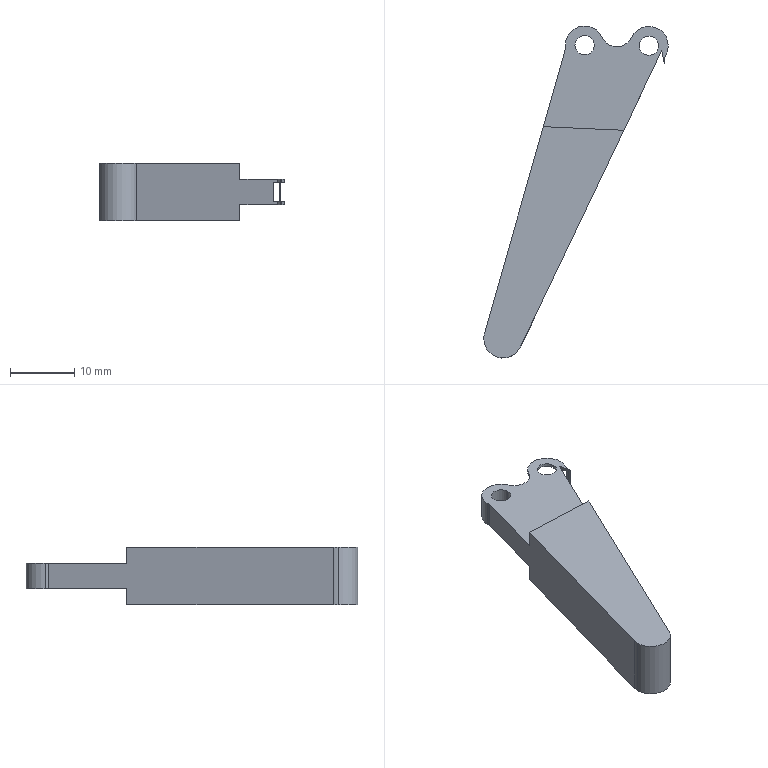Part | SolidWorks | features ICE 2, Extrusion 1, MirrorPattern 1, Scale 1 | 1 solid | 29 faces | box 28.674 x 51.63 x 9 mm | volume 3668 mm3 | cylinder 15 | plane 14 | commonest cylinder face diameters 3 x6 6 x6 4 x2 5 x1
STEP:
#1=CARTESIAN_POINT('',(-17.174,-2.918,4.));
#2=VERTEX_POINT('',#1);
#3=CARTESIAN_POINT('',(-17.133,-3.412,4.));
#4=VERTEX_POINT('',#3);
#5=CARTESIAN_POINT('',(-14.174,-2.918,4.));
#6=DIRECTION('',(0.,0.,1.));
#7=DIRECTION('',(1.,0.,0.));
#8=AXIS2_PLACEMENT_3D('',#5,#6,#7);
#9=CIRCLE('',#8,3.);
#10=EDGE_CURVE('',#2,#4,#9,.T.);
#11=ORIENTED_EDGE('',*,*,#10,.F.);
#12=CARTESIAN_POINT('',(-17.174,-2.918,0.));
#13=VERTEX_POINT('',#12);
#14=CARTESIAN_POINT('',(-17.174,-2.918,4.));
#15=DIRECTION('',(0.,0.,-1.));
#16=VECTOR('',#15,1000.);
#17=LINE('',#14,#16);
#18=EDGE_CURVE('',#2,#13,#17,.T.);
#19=ORIENTED_EDGE('',*,*,#18,.T.);
#20=CARTESIAN_POINT('',(-17.133,-3.412,0.));
#21=VERTEX_POINT('',#20);
#22=CARTESIAN_POINT('',(-14.174,-2.918,0.));
#23=DIRECTION('',(0.,0.,1.));
#24=DIRECTION('',(1.,0.,0.));
#25=AXIS2_PLACEMENT_3D('',#22,#23,#24);
#26=CIRCLE('',#25,3.);
#27=EDGE_CURVE('',#13,#21,#26,.T.);
#28=ORIENTED_EDGE('',*,*,#27,.T.);
#29=CARTESIAN_POINT('',(-17.133,-3.412,4.));
#30=DIRECTION('',(0.,0.,-1.));
#31=VECTOR('',#30,1000.);
#32=LINE('',#29,#31);
#33=EDGE_CURVE('',#4,#21,#32,.T.);
#34=ORIENTED_EDGE('',*,*,#33,.F.);
#35=EDGE_LOOP('',(#11,#19,#28,#34));
#36=FACE_OUTER_BOUND('',#35,.T.);
#37=CARTESIAN_POINT('',(-14.174,-2.918,4.));
#38=DIRECTION('',(0.,0.,-1.));
#39=DIRECTION('',(-1.,0.,0.));
#40=AXIS2_PLACEMENT_3D('',#37,#38,#39);
#41=CYLINDRICAL_SURFACE('',#40,3.);
#42=ADVANCED_FACE('',(#36),#41,.T.);
#43=CARTESIAN_POINT('',(-15.674,-2.918,4.));
#44=VERTEX_POINT('',#43);
#45=CARTESIAN_POINT('',(-12.674,-2.918,4.));
#46=VERTEX_POINT('',#45);
#47=CARTESIAN_POINT('',(-14.174,-2.918,4.));
#48=DIRECTION('',(0.,0.,1.));
#49=DIRECTION('',(1.,0.,0.));
#50=AXIS2_PLACEMENT_3D('',#47,#48,#49);
#51=CIRCLE('',#50,1.5);
#52=EDGE_CURVE('',#44,#46,#51,.T.);
#53=ORIENTED_EDGE('',*,*,#52,.T.);
#54=CARTESIAN_POINT('',(-12.674,-2.918,0.));
#55=VERTEX_POINT('',#54);
#56=CARTESIAN_POINT('',(-12.674,-2.918,4.));
#57=DIRECTION('',(0.,0.,-1.));
#58=VECTOR('',#57,1000.);
#59=LINE('',#56,#58);
#60=EDGE_CURVE('',#46,#55,#59,.T.);
#61=ORIENTED_EDGE('',*,*,#60,.T.);
#62=CARTESIAN_POINT('',(-15.674,-2.918,0.));
#63=VERTEX_POINT('',#62);
#64=CARTESIAN_POINT('',(-14.174,-2.918,0.));
#65=DIRECTION('',(0.,0.,1.));
#66=DIRECTION('',(1.,0.,0.));
#67=AXIS2_PLACEMENT_3D('',#64,#65,#66);
#68=CIRCLE('',#67,1.5);
#69=EDGE_CURVE('',#63,#55,#68,.T.);
#70=ORIENTED_EDGE('',*,*,#69,.F.);
#71=CARTESIAN_POINT('',(-15.674,-2.918,4.));
#72=DIRECTION('',(0.,0.,-1.));
#73=VECTOR('',#72,1000.);
#74=LINE('',#71,#73);
#75=EDGE_CURVE('',#44,#63,#74,.T.);
#76=ORIENTED_EDGE('',*,*,#75,.F.);
#77=EDGE_LOOP('',(#53,#61,#70,#76));
#78=FACE_OUTER_BOUND('',#77,.T.);
#79=CARTESIAN_POINT('',(-14.174,-2.918,4.));
#80=DIRECTION('',(0.,0.,-1.));
#81=DIRECTION('',(-1.,0.,0.));
#82=AXIS2_PLACEMENT_3D('',#79,#80,#81);
#83=CYLINDRICAL_SURFACE('',#82,1.5);
#84=ADVANCED_FACE('',(#78),#83,.F.);
#85=CARTESIAN_POINT('',(-29.848,-48.547,6.5));
#86=VERTEX_POINT('',#85);
#87=CARTESIAN_POINT('',(-24.14,-49.838,6.5));
#88=VERTEX_POINT('',#87);
#89=CARTESIAN_POINT('',(-26.848,-48.547,6.5));
#90=DIRECTION('',(0.,0.,1.));
#91=DIRECTION('',(1.,0.,0.));
#92=AXIS2_PLACEMENT_3D('',#89,#90,#91);
#93=CIRCLE('',#92,3.);
#94=EDGE_CURVE('',#86,#88,#93,.T.);
#95=ORIENTED_EDGE('',*,*,#94,.F.);
#96=CARTESIAN_POINT('',(-29.848,-48.547,-2.5));
#97=VERTEX_POINT('',#96);
#98=CARTESIAN_POINT('',(-29.848,-48.547,4.));
#99=DIRECTION('',(0.,0.,-1.));
#100=VECTOR('',#99,1000.);
#101=LINE('',#98,#100);
#102=EDGE_CURVE('',#86,#97,#101,.T.);
#103=ORIENTED_EDGE('',*,*,#102,.T.);
#104=CARTESIAN_POINT('',(-24.14,-49.838,-2.5));
#105=VERTEX_POINT('',#104);
#106=CARTESIAN_POINT('',(-26.848,-48.547,-2.5));
#107=DIRECTION('',(0.,0.,1.));
#108=DIRECTION('',(1.,0.,0.));
#109=AXIS2_PLACEMENT_3D('',#106,#107,#108);
#110=CIRCLE('',#109,3.);
#111=EDGE_CURVE('',#97,#105,#110,.T.);
#112=ORIENTED_EDGE('',*,*,#111,.T.);
#113=CARTESIAN_POINT('',(-24.14,-49.838,4.));
#114=DIRECTION('',(0.,0.,-1.));
#115=VECTOR('',#114,1000.);
#116=LINE('',#113,#115);
#117=EDGE_CURVE('',#88,#105,#116,.T.);
#118=ORIENTED_EDGE('',*,*,#117,.F.);
#119=EDGE_LOOP('',(#95,#103,#112,#118));
#120=FACE_OUTER_BOUND('',#119,.T.);
#121=CARTESIAN_POINT('',(-26.848,-48.547,4.));
#122=DIRECTION('',(0.,0.,-1.));
#123=DIRECTION('',(-1.,0.,0.));
#124=AXIS2_PLACEMENT_3D('',#121,#122,#123);
#125=CYLINDRICAL_SURFACE('',#124,3.);
#126=ADVANCED_FACE('',(#120),#125,.T.);
#127=CARTESIAN_POINT('',(-5.674,-2.989,0.5));
#128=VERTEX_POINT('',#127);
#129=CARTESIAN_POINT('',(-2.674,-2.989,0.5));
#130=VERTEX_POINT('',#129);
#131=CARTESIAN_POINT('',(-4.174,-2.989,0.5));
#132=DIRECTION('',(0.,0.,1.));
#133=DIRECTION('',(1.,0.,0.));
#134=AXIS2_PLACEMENT_3D('',#131,#132,#133);
#135=CIRCLE('',#134,1.5);
#136=EDGE_CURVE('',#128,#130,#135,.T.);
#137=ORIENTED_EDGE('',*,*,#136,.T.);
#138=CARTESIAN_POINT('',(-2.674,-2.989,0.));
#139=VERTEX_POINT('',#138);
#140=CARTESIAN_POINT('',(-2.674,-2.989,4.));
#141=DIRECTION('',(0.,0.,-1.));
#142=VECTOR('',#141,1000.);
#143=LINE('',#140,#142);
#144=EDGE_CURVE('',#130,#139,#143,.T.);
#145=ORIENTED_EDGE('',*,*,#144,.T.);
#146=CARTESIAN_POINT('',(-5.674,-2.989,0.));
#147=VERTEX_POINT('',#146);
#148=CARTESIAN_POINT('',(-4.174,-2.989,0.));
#149=DIRECTION('',(0.,0.,1.));
#150=DIRECTION('',(1.,0.,0.));
#151=AXIS2_PLACEMENT_3D('',#148,#149,#150);
#152=CIRCLE('',#151,1.5);
#153=EDGE_CURVE('',#147,#139,#152,.T.);
#154=ORIENTED_EDGE('',*,*,#153,.F.);
#155=CARTESIAN_POINT('',(-5.674,-2.989,4.));
#156=DIRECTION('',(0.,0.,-1.));
#157=VECTOR('',#156,1000.);
#158=LINE('',#155,#157);
#159=EDGE_CURVE('',#128,#147,#158,.T.);
#160=ORIENTED_EDGE('',*,*,#159,.F.);
#161=EDGE_LOOP('',(#137,#145,#154,#160));
#162=FACE_OUTER_BOUND('',#161,.T.);
#163=CARTESIAN_POINT('',(-4.174,-2.989,4.));
#164=DIRECTION('',(0.,0.,-1.));
#165=DIRECTION('',(-1.,0.,0.));
#166=AXIS2_PLACEMENT_3D('',#163,#164,#165);
#167=CYLINDRICAL_SURFACE('',#166,1.5);
#168=ADVANCED_FACE('',(#162),#167,.F.);
#169=CARTESIAN_POINT('',(-5.674,-2.989,4.));
#170=VERTEX_POINT('',#169);
#171=CARTESIAN_POINT('',(-2.674,-2.989,4.));
#172=VERTEX_POINT('',#171);
#173=CARTESIAN_POINT('',(-4.174,-2.989,4.));
#174=DIRECTION('',(0.,0.,1.));
#175=DIRECTION('',(1.,0.,0.));
#176=AXIS2_PLACEMENT_3D('',#173,#174,#175);
#177=CIRCLE('',#176,1.5);
#178=EDGE_CURVE('',#170,#172,#177,.T.);
#179=ORIENTED_EDGE('',*,*,#178,.T.);
#180=CARTESIAN_POINT('',(-2.674,-2.989,3.5));
#181=VERTEX_POINT('',#180);
#182=CARTESIAN_POINT('',(-2.674,-2.989,4.));
#183=DIRECTION('',(0.,0.,-1.));
#184=VECTOR('',#183,1000.);
#185=LINE('',#182,#184);
#186=EDGE_CURVE('',#172,#181,#185,.T.);
#187=ORIENTED_EDGE('',*,*,#186,.T.);
#188=CARTESIAN_POINT('',(-5.674,-2.989,3.5));
#189=VERTEX_POINT('',#188);
#190=CARTESIAN_POINT('',(-4.174,-2.989,3.5));
#191=DIRECTION('',(0.,0.,-1.));
#192=DIRECTION('',(-1.,0.,0.));
#193=AXIS2_PLACEMENT_3D('',#190,#191,#192);
#194=CIRCLE('',#193,1.5);
#195=EDGE_CURVE('',#181,#189,#194,.T.);
#196=ORIENTED_EDGE('',*,*,#195,.T.);
#197=CARTESIAN_POINT('',(-5.674,-2.989,4.));
#198=DIRECTION('',(0.,0.,-1.));
#199=VECTOR('',#198,1000.);
#200=LINE('',#197,#199);
#201=EDGE_CURVE('',#170,#189,#200,.T.);
#202=ORIENTED_EDGE('',*,*,#201,.F.);
#203=EDGE_LOOP('',(#179,#187,#196,#202));
#204=FACE_OUTER_BOUND('',#203,.T.);
#205=CARTESIAN_POINT('',(-4.174,-2.989,4.));
#206=DIRECTION('',(0.,0.,-1.));
#207=DIRECTION('',(-1.,0.,0.));
#208=AXIS2_PLACEMENT_3D('',#205,#206,#207);
#209=CYLINDRICAL_SURFACE('',#208,1.5);
#210=ADVANCED_FACE('',(#204),#209,.F.);
#211=CARTESIAN_POINT('',(-1.828,-5.461,4.));
#212=VERTEX_POINT('',#211);
#213=CARTESIAN_POINT('',(-1.566,-4.473,4.));
#214=VERTEX_POINT('',#213);
#215=CARTESIAN_POINT('',(0.1723,-5.461,4.));
#216=DIRECTION('',(0.,0.,-1.));
#217=DIRECTION('',(1.,0.,0.));
#218=AXIS2_PLACEMENT_3D('',#215,#216,#217);
#219=CIRCLE('',#218,2.);
#220=EDGE_CURVE('',#212,#214,#219,.T.);
#221=ORIENTED_EDGE('',*,*,#220,.F.);
#222=CARTESIAN_POINT('',(-1.828,-5.461,0.));
#223=VERTEX_POINT('',#222);
#224=CARTESIAN_POINT('',(-1.828,-5.461,4.));
#225=DIRECTION('',(0.,0.,-1.));
#226=VECTOR('',#225,1000.);
#227=LINE('',#224,#226);
#228=EDGE_CURVE('',#212,#223,#227,.T.);
#229=ORIENTED_EDGE('',*,*,#228,.T.);
#230=CARTESIAN_POINT('',(-1.566,-4.473,0.));
#231=VERTEX_POINT('',#230);
#232=CARTESIAN_POINT('',(0.1723,-5.461,0.));
#233=DIRECTION('',(0.,0.,-1.));
#234=DIRECTION('',(1.,0.,0.));
#235=AXIS2_PLACEMENT_3D('',#232,#233,#234);
#236=CIRCLE('',#235,2.);
#237=EDGE_CURVE('',#223,#231,#236,.T.);
#238=ORIENTED_EDGE('',*,*,#237,.T.);
#239=CARTESIAN_POINT('',(-1.566,-4.473,0.5));
#240=VERTEX_POINT('',#239);
#241=CARTESIAN_POINT('',(-1.566,-4.473,4.));
#242=DIRECTION('',(0.,0.,-1.));
#243=VECTOR('',#242,1000.);
#244=LINE('',#241,#243);
#245=EDGE_CURVE('',#240,#231,#244,.T.);
#246=ORIENTED_EDGE('',*,*,#245,.F.);
#247=CARTESIAN_POINT('',(-1.774,-5.,0.5));
#248=VERTEX_POINT('',#247);
#249=CARTESIAN_POINT('',(0.1723,-5.461,0.5));
#250=DIRECTION('',(0.,0.,-1.));
#251=DIRECTION('',(1.,0.,0.));
#252=AXIS2_PLACEMENT_3D('',#249,#250,#251);
#253=CIRCLE('',#252,2.);
#254=EDGE_CURVE('',#248,#240,#253,.T.);
#255=ORIENTED_EDGE('',*,*,#254,.F.);
#256=CARTESIAN_POINT('',(-1.774,-5.,3.5));
#257=VERTEX_POINT('',#256);
#258=CARTESIAN_POINT('',(-1.774,-5.,4.));
#259=DIRECTION('',(0.,0.,1.));
#260=VECTOR('',#259,1000.);
#261=LINE('',#258,#260);
#262=EDGE_CURVE('',#248,#257,#261,.T.);
#263=ORIENTED_EDGE('',*,*,#262,.T.);
#264=CARTESIAN_POINT('',(-1.566,-4.473,3.5));
#265=VERTEX_POINT('',#264);
#266=CARTESIAN_POINT('',(0.1723,-5.461,3.5));
#267=DIRECTION('',(0.,0.,1.));
#268=DIRECTION('',(-1.,0.,0.));
#269=AXIS2_PLACEMENT_3D('',#266,#267,#268);
#270=CIRCLE('',#269,2.);
#271=EDGE_CURVE('',#265,#257,#270,.T.);
#272=ORIENTED_EDGE('',*,*,#271,.F.);
#273=CARTESIAN_POINT('',(-1.566,-4.473,4.));
#274=DIRECTION('',(0.,0.,-1.));
#275=VECTOR('',#274,1000.);
#276=LINE('',#273,#275);
#277=EDGE_CURVE('',#214,#265,#276,.T.);
#278=ORIENTED_EDGE('',*,*,#277,.F.);
#279=EDGE_LOOP('',(#221,#229,#238,#246,#255,#263,#272,#278));
#280=FACE_OUTER_BOUND('',#279,.T.);
#281=CARTESIAN_POINT('',(0.1723,-5.461,4.));
#282=DIRECTION('',(0.,0.,-1.));
#283=DIRECTION('',(-1.,0.,0.));
#284=AXIS2_PLACEMENT_3D('',#281,#282,#283);
#285=CYLINDRICAL_SURFACE('',#284,2.);
#286=ADVANCED_FACE('',(#280),#285,.F.);
#287=CARTESIAN_POINT('',(-2.769,-5.,3.5));
#288=VERTEX_POINT('',#287);
#289=CARTESIAN_POINT('',(-2.769,-5.,0.5));
#290=VERTEX_POINT('',#289);
#291=CARTESIAN_POINT('',(-2.769,-5.,4.));
#292=DIRECTION('',(0.,0.,-1.));
#293=VECTOR('',#292,1000.);
#294=LINE('',#291,#293);
#295=EDGE_CURVE('',#288,#290,#294,.T.);
#296=ORIENTED_EDGE('',*,*,#295,.F.);
#297=CARTESIAN_POINT('',(-2.173,-3.748,3.5));
#298=VERTEX_POINT('',#297);
#299=CARTESIAN_POINT('',(-0.3148,0.15,3.5));
#300=DIRECTION('',(0.4302,0.9027,0.));
#301=VECTOR('',#300,1000.);
#302=LINE('',#299,#301);
#303=EDGE_CURVE('',#288,#298,#302,.T.);
#304=ORIENTED_EDGE('',*,*,#303,.T.);
#305=CARTESIAN_POINT('',(-2.173,-3.748,4.));
#306=VERTEX_POINT('',#305);
#307=CARTESIAN_POINT('',(-2.173,-3.748,4.));
#308=DIRECTION('',(0.,0.,-1.));
#309=VECTOR('',#308,1000.);
#310=LINE('',#307,#309);
#311=EDGE_CURVE('',#306,#298,#310,.T.);
#312=ORIENTED_EDGE('',*,*,#311,.F.);
#313=CARTESIAN_POINT('',(-8.079,-16.141,4.));
#314=VERTEX_POINT('',#313);
#315=CARTESIAN_POINT('',(-0.3148,0.15,4.));
#316=DIRECTION('',(-0.4302,-0.9027,0.));
#317=VECTOR('',#316,1000.);
#318=LINE('',#315,#317);
#319=EDGE_CURVE('',#306,#314,#318,.T.);
#320=ORIENTED_EDGE('',*,*,#319,.T.);
#321=CARTESIAN_POINT('',(-8.079,-16.141,6.5));
#322=VERTEX_POINT('',#321);
#323=CARTESIAN_POINT('',(-8.079,-16.141,6.5));
#324=DIRECTION('',(0.,0.,-1.));
#325=VECTOR('',#324,1000.);
#326=LINE('',#323,#325);
#327=EDGE_CURVE('',#322,#314,#326,.T.);
#328=ORIENTED_EDGE('',*,*,#327,.F.);
#329=CARTESIAN_POINT('',(-24.14,-49.838,6.5));
#330=DIRECTION('',(0.4302,0.9027,0.));
#331=VECTOR('',#330,1000.);
#332=LINE('',#329,#331);
#333=EDGE_CURVE('',#88,#322,#332,.T.);
#334=ORIENTED_EDGE('',*,*,#333,.F.);
#335=ORIENTED_EDGE('',*,*,#117,.T.);
#336=CARTESIAN_POINT('',(-8.079,-16.141,-2.5));
#337=VERTEX_POINT('',#336);
#338=CARTESIAN_POINT('',(-24.14,-49.838,-2.5));
#339=DIRECTION('',(0.4302,0.9027,0.));
#340=VECTOR('',#339,1000.);
#341=LINE('',#338,#340);
#342=EDGE_CURVE('',#105,#337,#341,.T.);
#343=ORIENTED_EDGE('',*,*,#342,.T.);
#344=CARTESIAN_POINT('',(-8.079,-16.141,0.));
#345=VERTEX_POINT('',#344);
#346=CARTESIAN_POINT('',(-8.079,-16.141,-2.5));
#347=DIRECTION('',(0.,0.,1.));
#348=VECTOR('',#347,1000.);
#349=LINE('',#346,#348);
#350=EDGE_CURVE('',#337,#345,#349,.T.);
#351=ORIENTED_EDGE('',*,*,#350,.T.);
#352=CARTESIAN_POINT('',(-2.173,-3.748,0.));
#353=VERTEX_POINT('',#352);
#354=CARTESIAN_POINT('',(-0.3148,0.15,0.));
#355=DIRECTION('',(-0.4302,-0.9027,0.));
#356=VECTOR('',#355,1000.);
#357=LINE('',#354,#356);
#358=EDGE_CURVE('',#353,#345,#357,.T.);
#359=ORIENTED_EDGE('',*,*,#358,.F.);
#360=CARTESIAN_POINT('',(-2.173,-3.748,0.5));
#361=VERTEX_POINT('',#360);
#362=CARTESIAN_POINT('',(-2.173,-3.748,4.));
#363=DIRECTION('',(0.,0.,-1.));
#364=VECTOR('',#363,1000.);
#365=LINE('',#362,#364);
#366=EDGE_CURVE('',#361,#353,#365,.T.);
#367=ORIENTED_EDGE('',*,*,#366,.F.);
#368=CARTESIAN_POINT('',(-0.3148,0.15,0.5));
#369=DIRECTION('',(-0.4302,-0.9027,0.));
#370=VECTOR('',#369,1000.);
#371=LINE('',#368,#370);
#372=EDGE_CURVE('',#361,#290,#371,.T.);
#373=ORIENTED_EDGE('',*,*,#372,.T.);
#374=EDGE_LOOP('',(#296,#304,#312,#320,#328,#334,#335,#343,#351,#359,#367,#373));
#375=FACE_OUTER_BOUND('',#374,.T.);
#376=CARTESIAN_POINT('',(-0.3148,0.15,4.));
#377=DIRECTION('',(0.9027,-0.4302,0.));
#378=DIRECTION('',(0.4302,0.9027,0.));
#379=AXIS2_PLACEMENT_3D('',#376,#377,#378);
#380=PLANE('',#379);
#381=ADVANCED_FACE('',(#375),#380,.T.);
#382=ORIENTED_EDGE('',*,*,#311,.T.);
#383=CARTESIAN_POINT('',(-1.945,-5.,3.5));
#384=VERTEX_POINT('',#383);
#385=CARTESIAN_POINT('',(-2.764,-0.5035,3.5));
#386=DIRECTION('',(0.1792,-0.9838,0.));
#387=VECTOR('',#386,1000.);
#388=LINE('',#385,#387);
#389=EDGE_CURVE('',#298,#384,#388,.T.);
#390=ORIENTED_EDGE('',*,*,#389,.T.);
#391=CARTESIAN_POINT('',(-1.945,-5.,0.5));
#392=VERTEX_POINT('',#391);
#393=CARTESIAN_POINT('',(-1.945,-5.,4.));
#394=DIRECTION('',(0.,0.,1.));
#395=VECTOR('',#394,1000.);
#396=LINE('',#393,#395);
#397=EDGE_CURVE('',#392,#384,#396,.T.);
#398=ORIENTED_EDGE('',*,*,#397,.F.);
#399=CARTESIAN_POINT('',(-2.764,-0.5035,0.5));
#400=DIRECTION('',(-0.1792,0.9838,0.));
#401=VECTOR('',#400,1000.);
#402=LINE('',#399,#401);
#403=EDGE_CURVE('',#392,#361,#402,.T.);
#404=ORIENTED_EDGE('',*,*,#403,.T.);
#405=ORIENTED_EDGE('',*,*,#366,.T.);
#406=CARTESIAN_POINT('',(-1.795,-5.82,0.));
#407=VERTEX_POINT('',#406);
#408=CARTESIAN_POINT('',(-2.764,-0.5035,0.));
#409=DIRECTION('',(-0.1792,0.9838,0.));
#410=VECTOR('',#409,1000.);
#411=LINE('',#408,#410);
#412=EDGE_CURVE('',#407,#353,#411,.T.);
#413=ORIENTED_EDGE('',*,*,#412,.F.);
#414=CARTESIAN_POINT('',(-1.795,-5.82,4.));
#415=VERTEX_POINT('',#414);
#416=CARTESIAN_POINT('',(-1.795,-5.82,4.));
#417=DIRECTION('',(0.,0.,-1.));
#418=VECTOR('',#417,1000.);
#419=LINE('',#416,#418);
#420=EDGE_CURVE('',#415,#407,#419,.T.);
#421=ORIENTED_EDGE('',*,*,#420,.F.);
#422=CARTESIAN_POINT('',(-2.764,-0.5035,4.));
#423=DIRECTION('',(-0.1792,0.9838,0.));
#424=VECTOR('',#423,1000.);
#425=LINE('',#422,#424);
#426=EDGE_CURVE('',#415,#306,#425,.T.);
#427=ORIENTED_EDGE('',*,*,#426,.T.);
#428=EDGE_LOOP('',(#382,#390,#398,#404,#405,#413,#421,#427));
#429=FACE_OUTER_BOUND('',#428,.T.);
#430=CARTESIAN_POINT('',(-2.764,-0.5035,4.));
#431=DIRECTION('',(-0.9838,-0.1792,0.));
#432=DIRECTION('',(0.1792,-0.9838,0.));
#433=AXIS2_PLACEMENT_3D('',#430,#431,#432);
#434=PLANE('',#433);
#435=ADVANCED_FACE('',(#429),#434,.T.);
#436=ORIENTED_EDGE('',*,*,#228,.F.);
#437=CARTESIAN_POINT('',(0.1723,-5.461,4.));
#438=DIRECTION('',(0.,0.,-1.));
#439=DIRECTION('',(1.,0.,0.));
#440=AXIS2_PLACEMENT_3D('',#437,#438,#439);
#441=CIRCLE('',#440,2.);
#442=EDGE_CURVE('',#415,#212,#441,.T.);
#443=ORIENTED_EDGE('',*,*,#442,.F.);
#444=ORIENTED_EDGE('',*,*,#420,.T.);
#445=CARTESIAN_POINT('',(0.1723,-5.461,0.));
#446=DIRECTION('',(0.,0.,-1.));
#447=DIRECTION('',(1.,0.,0.));
#448=AXIS2_PLACEMENT_3D('',#445,#446,#447);
#449=CIRCLE('',#448,2.);
#450=EDGE_CURVE('',#407,#223,#449,.T.);
#451=ORIENTED_EDGE('',*,*,#450,.T.);
#452=EDGE_LOOP('',(#436,#443,#444,#451));
#453=FACE_OUTER_BOUND('',#452,.T.);
#454=CARTESIAN_POINT('',(0.1723,-5.461,4.));
#455=DIRECTION('',(0.,0.,-1.));
#456=DIRECTION('',(-1.,0.,0.));
#457=AXIS2_PLACEMENT_3D('',#454,#455,#456);
#458=CYLINDRICAL_SURFACE('',#457,2.);
#459=ADVANCED_FACE('',(#453),#458,.F.);
#460=CARTESIAN_POINT('',(-6.892,-1.72,3.5));
#461=VERTEX_POINT('',#460);
#462=CARTESIAN_POINT('',(-4.174,-2.989,3.5));
#463=DIRECTION('',(0.,0.,-1.));
#464=DIRECTION('',(-1.,0.,0.));
#465=AXIS2_PLACEMENT_3D('',#462,#463,#464);
#466=CIRCLE('',#465,3.);
#467=EDGE_CURVE('',#461,#265,#466,.T.);
#468=ORIENTED_EDGE('',*,*,#467,.F.);
#469=CARTESIAN_POINT('',(-6.892,-1.72,4.));
#470=VERTEX_POINT('',#469);
#471=CARTESIAN_POINT('',(-6.892,-1.72,4.));
#472=DIRECTION('',(0.,0.,-1.));
#473=VECTOR('',#472,1000.);
#474=LINE('',#471,#473);
#475=EDGE_CURVE('',#470,#461,#474,.T.);
#476=ORIENTED_EDGE('',*,*,#475,.F.);
#477=CARTESIAN_POINT('',(-4.174,-2.989,4.));
#478=DIRECTION('',(0.,0.,1.));
#479=DIRECTION('',(1.,0.,0.));
#480=AXIS2_PLACEMENT_3D('',#477,#478,#479);
#481=CIRCLE('',#480,3.);
#482=EDGE_CURVE('',#214,#470,#481,.T.);
#483=ORIENTED_EDGE('',*,*,#482,.F.);
#484=ORIENTED_EDGE('',*,*,#277,.T.);
#485=EDGE_LOOP('',(#468,#476,#483,#484));
#486=FACE_OUTER_BOUND('',#485,.T.);
#487=CARTESIAN_POINT('',(-4.174,-2.989,4.));
#488=DIRECTION('',(0.,0.,-1.));
#489=DIRECTION('',(-1.,0.,0.));
#490=AXIS2_PLACEMENT_3D('',#487,#488,#489);
#491=CYLINDRICAL_SURFACE('',#490,3.);
#492=ADVANCED_FACE('',(#486),#491,.T.);
#493=CARTESIAN_POINT('',(-6.892,-1.72,0.5));
#494=VERTEX_POINT('',#493);
#495=CARTESIAN_POINT('',(-4.174,-2.989,0.5));
#496=DIRECTION('',(0.,0.,1.));
#497=DIRECTION('',(1.,0.,0.));
#498=AXIS2_PLACEMENT_3D('',#495,#496,#497);
#499=CIRCLE('',#498,3.);
#500=EDGE_CURVE('',#240,#494,#499,.T.);
#501=ORIENTED_EDGE('',*,*,#500,.F.);
#502=ORIENTED_EDGE('',*,*,#245,.T.);
#503=CARTESIAN_POINT('',(-6.892,-1.72,0.));
#504=VERTEX_POINT('',#503);
#505=CARTESIAN_POINT('',(-4.174,-2.989,0.));
#506=DIRECTION('',(0.,0.,1.));
#507=DIRECTION('',(1.,0.,0.));
#508=AXIS2_PLACEMENT_3D('',#505,#506,#507);
#509=CIRCLE('',#508,3.);
#510=EDGE_CURVE('',#231,#504,#509,.T.);
#511=ORIENTED_EDGE('',*,*,#510,.T.);
#512=CARTESIAN_POINT('',(-6.892,-1.72,4.));
#513=DIRECTION('',(0.,0.,-1.));
#514=VECTOR('',#513,1000.);
#515=LINE('',#512,#514);
#516=EDGE_CURVE('',#494,#504,#515,.T.);
#517=ORIENTED_EDGE('',*,*,#516,.F.);
#518=EDGE_LOOP('',(#501,#502,#511,#517));
#519=FACE_OUTER_BOUND('',#518,.T.);
#520=CARTESIAN_POINT('',(-4.174,-2.989,4.));
#521=DIRECTION('',(0.,0.,-1.));
#522=DIRECTION('',(-1.,0.,0.));
#523=AXIS2_PLACEMENT_3D('',#520,#521,#522);
#524=CYLINDRICAL_SURFACE('',#523,3.);
#525=ADVANCED_FACE('',(#519),#524,.T.);
#526=ORIENTED_EDGE('',*,*,#475,.T.);
#527=CARTESIAN_POINT('',(-8.674,-3.115,3.5));
#528=VERTEX_POINT('',#527);
#529=CARTESIAN_POINT('',(-9.157,-0.6624,3.5));
#530=DIRECTION('',(0.,0.,-1.));
#531=DIRECTION('',(-1.,0.,0.));
#532=AXIS2_PLACEMENT_3D('',#529,#530,#531);
#533=CIRCLE('',#532,2.5);
#534=EDGE_CURVE('',#461,#528,#533,.T.);
#535=ORIENTED_EDGE('',*,*,#534,.T.);
#536=CARTESIAN_POINT('',(-8.674,-3.115,0.5));
#537=VERTEX_POINT('',#536);
#538=CARTESIAN_POINT('',(-8.674,-3.115,4.));
#539=DIRECTION('',(0.,0.,-1.));
#540=VECTOR('',#539,1000.);
#541=LINE('',#538,#540);
#542=EDGE_CURVE('',#528,#537,#541,.T.);
#543=ORIENTED_EDGE('',*,*,#542,.T.);
#544=CARTESIAN_POINT('',(-9.157,-0.6624,0.5));
#545=DIRECTION('',(0.,0.,1.));
#546=DIRECTION('',(1.,0.,0.));
#547=AXIS2_PLACEMENT_3D('',#544,#545,#546);
#548=CIRCLE('',#547,2.5);
#549=EDGE_CURVE('',#537,#494,#548,.T.);
#550=ORIENTED_EDGE('',*,*,#549,.T.);
#551=ORIENTED_EDGE('',*,*,#516,.T.);
#552=CARTESIAN_POINT('',(-11.438,-1.688,0.));
#553=VERTEX_POINT('',#552);
#554=CARTESIAN_POINT('',(-9.157,-0.6624,0.));
#555=DIRECTION('',(0.,0.,1.));
#556=DIRECTION('',(1.,0.,0.));
#557=AXIS2_PLACEMENT_3D('',#554,#555,#556);
#558=CIRCLE('',#557,2.5);
#559=EDGE_CURVE('',#553,#504,#558,.T.);
#560=ORIENTED_EDGE('',*,*,#559,.F.);
#561=CARTESIAN_POINT('',(-11.438,-1.688,4.));
#562=VERTEX_POINT('',#561);
#563=CARTESIAN_POINT('',(-11.438,-1.688,4.));
#564=DIRECTION('',(0.,0.,-1.));
#565=VECTOR('',#564,1000.);
#566=LINE('',#563,#565);
#567=EDGE_CURVE('',#562,#553,#566,.T.);
#568=ORIENTED_EDGE('',*,*,#567,.F.);
#569=CARTESIAN_POINT('',(-9.157,-0.6624,4.));
#570=DIRECTION('',(0.,0.,1.));
#571=DIRECTION('',(1.,0.,0.));
#572=AXIS2_PLACEMENT_3D('',#569,#570,#571);
#573=CIRCLE('',#572,2.5);
#574=EDGE_CURVE('',#562,#470,#573,.T.);
#575=ORIENTED_EDGE('',*,*,#574,.T.);
#576=EDGE_LOOP('',(#526,#535,#543,#550,#551,#560,#568,#575));
#577=FACE_OUTER_BOUND('',#576,.T.);
#578=CARTESIAN_POINT('',(-9.157,-0.6624,4.));
#579=DIRECTION('',(0.,0.,-1.));
#580=DIRECTION('',(-1.,0.,0.));
#581=AXIS2_PLACEMENT_3D('',#578,#579,#580);
#582=CYLINDRICAL_SURFACE('',#581,2.5);
#583=ADVANCED_FACE('',(#577),#582,.F.);
#584=ORIENTED_EDGE('',*,*,#186,.F.);
#585=CARTESIAN_POINT('',(-4.174,-2.989,4.));
#586=DIRECTION('',(0.,0.,1.));
#587=DIRECTION('',(1.,0.,0.));
#588=AXIS2_PLACEMENT_3D('',#585,#586,#587);
#589=CIRCLE('',#588,1.5);
#590=EDGE_CURVE('',#172,#170,#589,.T.);
#591=ORIENTED_EDGE('',*,*,#590,.T.);
#592=ORIENTED_EDGE('',*,*,#201,.T.);
#593=CARTESIAN_POINT('',(-4.174,-2.989,3.5));
#594=DIRECTION('',(0.,0.,-1.));
#595=DIRECTION('',(-1.,0.,0.));
#596=AXIS2_PLACEMENT_3D('',#593,#594,#595);
#597=CIRCLE('',#596,1.5);
#598=EDGE_CURVE('',#189,#181,#597,.T.);
#599=ORIENTED_EDGE('',*,*,#598,.T.);
#600=EDGE_LOOP('',(#584,#591,#592,#599));
#601=FACE_OUTER_BOUND('',#600,.T.);
#602=CARTESIAN_POINT('',(-4.174,-2.989,4.));
#603=DIRECTION('',(0.,0.,-1.));
#604=DIRECTION('',(-1.,0.,0.));
#605=AXIS2_PLACEMENT_3D('',#602,#603,#604);
#606=CYLINDRICAL_SURFACE('',#605,1.5);
#607=ADVANCED_FACE('',(#601),#606,.F.);
#608=ORIENTED_EDGE('',*,*,#144,.F.);
#609=CARTESIAN_POINT('',(-4.174,-2.989,0.5));
#610=DIRECTION('',(0.,0.,1.));
#611=DIRECTION('',(1.,0.,0.));
#612=AXIS2_PLACEMENT_3D('',#609,#610,#611);
#613=CIRCLE('',#612,1.5);
#614=EDGE_CURVE('',#130,#128,#613,.T.);
#615=ORIENTED_EDGE('',*,*,#614,.T.);
#616=ORIENTED_EDGE('',*,*,#159,.T.);
#617=CARTESIAN_POINT('',(-4.174,-2.989,0.));
#618=DIRECTION('',(0.,0.,1.));
#619=DIRECTION('',(1.,0.,0.));
#620=AXIS2_PLACEMENT_3D('',#617,#618,#619);
#621=CIRCLE('',#620,1.5);
#622=EDGE_CURVE('',#139,#147,#621,.T.);
#623=ORIENTED_EDGE('',*,*,#622,.F.);
#624=EDGE_LOOP('',(#608,#615,#616,#623));
#625=FACE_OUTER_BOUND('',#624,.T.);
#626=CARTESIAN_POINT('',(-4.174,-2.989,4.));
#627=DIRECTION('',(0.,0.,-1.));
#628=DIRECTION('',(-1.,0.,0.));
#629=AXIS2_PLACEMENT_3D('',#626,#627,#628);
#630=CYLINDRICAL_SURFACE('',#629,1.5);
#631=ADVANCED_FACE('',(#625),#630,.F.);
#632=CARTESIAN_POINT('',(-20.595,-15.587,0.));
#633=VERTEX_POINT('',#632);
#634=CARTESIAN_POINT('',(-14.953,4.252,0.));
#635=DIRECTION('',(0.2735,0.9619,0.));
#636=VECTOR('',#635,1000.);
#637=LINE('',#634,#636);
#638=EDGE_CURVE('',#633,#21,#637,.T.);
#639=ORIENTED_EDGE('',*,*,#638,.F.);
#640=CARTESIAN_POINT('',(-20.595,-15.587,-2.5));
#641=VERTEX_POINT('',#640);
#642=CARTESIAN_POINT('',(-20.595,-15.587,-2.5));
#643=DIRECTION('',(0.,0.,1.));
#644=VECTOR('',#643,1000.);
#645=LINE('',#642,#644);
#646=EDGE_CURVE('',#641,#633,#645,.T.);
#647=ORIENTED_EDGE('',*,*,#646,.F.);
#648=CARTESIAN_POINT('',(-29.733,-47.727,-2.5));
#649=VERTEX_POINT('',#648);
#650=CARTESIAN_POINT('',(-20.595,-15.587,-2.5));
#651=DIRECTION('',(-0.2735,-0.9619,0.));
#652=VECTOR('',#651,1000.);
#653=LINE('',#650,#652);
#654=EDGE_CURVE('',#641,#649,#653,.T.);
#655=ORIENTED_EDGE('',*,*,#654,.T.);
#656=CARTESIAN_POINT('',(-29.733,-47.727,6.5));
#657=VERTEX_POINT('',#656);
#658=CARTESIAN_POINT('',(-29.733,-47.727,4.));
#659=DIRECTION('',(0.,0.,-1.));
#660=VECTOR('',#659,1000.);
#661=LINE('',#658,#660);
#662=EDGE_CURVE('',#657,#649,#661,.T.);
#663=ORIENTED_EDGE('',*,*,#662,.F.);
#664=CARTESIAN_POINT('',(-20.595,-15.587,6.5));
#665=VERTEX_POINT('',#664);
#666=CARTESIAN_POINT('',(-20.595,-15.587,6.5));
#667=DIRECTION('',(-0.2735,-0.9619,0.));
#668=VECTOR('',#667,1000.);
#669=LINE('',#666,#668);
#670=EDGE_CURVE('',#665,#657,#669,.T.);
#671=ORIENTED_EDGE('',*,*,#670,.F.);
#672=CARTESIAN_POINT('',(-20.595,-15.587,4.));
#673=VERTEX_POINT('',#672);
#674=CARTESIAN_POINT('',(-20.595,-15.587,6.5));
#675=DIRECTION('',(0.,0.,-1.));
#676=VECTOR('',#675,1000.);
#677=LINE('',#674,#676);
#678=EDGE_CURVE('',#665,#673,#677,.T.);
#679=ORIENTED_EDGE('',*,*,#678,.T.);
#680=CARTESIAN_POINT('',(-14.953,4.252,4.));
#681=DIRECTION('',(0.2735,0.9619,0.));
#682=VECTOR('',#681,1000.);
#683=LINE('',#680,#682);
#684=EDGE_CURVE('',#673,#4,#683,.T.);
#685=ORIENTED_EDGE('',*,*,#684,.T.);
#686=ORIENTED_EDGE('',*,*,#33,.T.);
#687=EDGE_LOOP('',(#639,#647,#655,#663,#671,#679,#685,#686));
#688=FACE_OUTER_BOUND('',#687,.T.);
#689=CARTESIAN_POINT('',(-14.953,4.252,4.));
#690=DIRECTION('',(-0.9619,0.2735,0.));
#691=DIRECTION('',(-0.2735,-0.9619,0.));
#692=AXIS2_PLACEMENT_3D('',#689,#690,#691);
#693=PLANE('',#692);
#694=ADVANCED_FACE('',(#688),#693,.T.);
#695=ORIENTED_EDGE('',*,*,#102,.F.);
#696=CARTESIAN_POINT('',(-26.848,-48.547,6.5));
#697=DIRECTION('',(0.,0.,1.));
#698=DIRECTION('',(1.,0.,0.));
#699=AXIS2_PLACEMENT_3D('',#696,#697,#698);
#700=CIRCLE('',#699,3.);
#701=EDGE_CURVE('',#657,#86,#700,.T.);
#702=ORIENTED_EDGE('',*,*,#701,.F.);
#703=ORIENTED_EDGE('',*,*,#662,.T.);
#704=CARTESIAN_POINT('',(-26.848,-48.547,-2.5));
#705=DIRECTION('',(0.,0.,1.));
#706=DIRECTION('',(1.,0.,0.));
#707=AXIS2_PLACEMENT_3D('',#704,#705,#706);
#708=CIRCLE('',#707,3.);
#709=EDGE_CURVE('',#649,#97,#708,.T.);
#710=ORIENTED_EDGE('',*,*,#709,.T.);
#711=EDGE_LOOP('',(#695,#702,#703,#710));
#712=FACE_OUTER_BOUND('',#711,.T.);
#713=CARTESIAN_POINT('',(-26.848,-48.547,4.));
#714=DIRECTION('',(0.,0.,-1.));
#715=DIRECTION('',(-1.,0.,0.));
#716=AXIS2_PLACEMENT_3D('',#713,#714,#715);
#717=CYLINDRICAL_SURFACE('',#716,3.);
#718=ADVANCED_FACE('',(#712),#717,.T.);
#719=ORIENTED_EDGE('',*,*,#60,.F.);
#720=CARTESIAN_POINT('',(-14.174,-2.918,4.));
#721=DIRECTION('',(0.,0.,1.));
#722=DIRECTION('',(1.,0.,0.));
#723=AXIS2_PLACEMENT_3D('',#720,#721,#722);
#724=CIRCLE('',#723,1.5);
#725=EDGE_CURVE('',#46,#44,#724,.T.);
#726=ORIENTED_EDGE('',*,*,#725,.T.);
#727=ORIENTED_EDGE('',*,*,#75,.T.);
#728=CARTESIAN_POINT('',(-14.174,-2.918,0.));
#729=DIRECTION('',(0.,0.,1.));
#730=DIRECTION('',(1.,0.,0.));
#731=AXIS2_PLACEMENT_3D('',#728,#729,#730);
#732=CIRCLE('',#731,1.5);
#733=EDGE_CURVE('',#55,#63,#732,.T.);
#734=ORIENTED_EDGE('',*,*,#733,.F.);
#735=EDGE_LOOP('',(#719,#726,#727,#734));
#736=FACE_OUTER_BOUND('',#735,.T.);
#737=CARTESIAN_POINT('',(-14.174,-2.918,4.));
#738=DIRECTION('',(0.,0.,-1.));
#739=DIRECTION('',(-1.,0.,0.));
#740=AXIS2_PLACEMENT_3D('',#737,#738,#739);
#741=CYLINDRICAL_SURFACE('',#740,1.5);
#742=ADVANCED_FACE('',(#736),#741,.F.);
#743=ORIENTED_EDGE('',*,*,#18,.F.);
#744=CARTESIAN_POINT('',(-14.174,-2.918,4.));
#745=DIRECTION('',(0.,0.,1.));
#746=DIRECTION('',(1.,0.,0.));
#747=AXIS2_PLACEMENT_3D('',#744,#745,#746);
#748=CIRCLE('',#747,3.);
#749=EDGE_CURVE('',#562,#2,#748,.T.);
#750=ORIENTED_EDGE('',*,*,#749,.F.);
#751=ORIENTED_EDGE('',*,*,#567,.T.);
#752=CARTESIAN_POINT('',(-14.174,-2.918,0.));
#753=DIRECTION('',(0.,0.,1.));
#754=DIRECTION('',(1.,0.,0.));
#755=AXIS2_PLACEMENT_3D('',#752,#753,#754);
#756=CIRCLE('',#755,3.);
#757=EDGE_CURVE('',#553,#13,#756,.T.);
#758=ORIENTED_EDGE('',*,*,#757,.T.);
#759=EDGE_LOOP('',(#743,#750,#751,#758));
#760=FACE_OUTER_BOUND('',#759,.T.);
#761=CARTESIAN_POINT('',(-14.174,-2.918,4.));
#762=DIRECTION('',(0.,0.,-1.));
#763=DIRECTION('',(-1.,0.,0.));
#764=AXIS2_PLACEMENT_3D('',#761,#762,#763);
#765=CYLINDRICAL_SURFACE('',#764,3.);
#766=ADVANCED_FACE('',(#760),#765,.T.);
#767=CARTESIAN_POINT('',(-8.079,-16.141,4.));
#768=DIRECTION('',(-0.999,0.04422,0.));
#769=VECTOR('',#768,1000.);
#770=LINE('',#767,#769);
#771=EDGE_CURVE('',#314,#673,#770,.T.);
#772=ORIENTED_EDGE('',*,*,#771,.F.);
#773=ORIENTED_EDGE('',*,*,#319,.F.);
#774=ORIENTED_EDGE('',*,*,#426,.F.);
#775=ORIENTED_EDGE('',*,*,#442,.T.);
#776=ORIENTED_EDGE('',*,*,#220,.T.);
#777=ORIENTED_EDGE('',*,*,#482,.T.);
#778=ORIENTED_EDGE('',*,*,#574,.F.);
#779=ORIENTED_EDGE('',*,*,#749,.T.);
#780=ORIENTED_EDGE('',*,*,#10,.T.);
#781=ORIENTED_EDGE('',*,*,#684,.F.);
#782=EDGE_LOOP('',(#772,#773,#774,#775,#776,#777,#778,#779,#780,#781));
#783=FACE_OUTER_BOUND('',#782,.T.);
#784=ORIENTED_EDGE('',*,*,#52,.F.);
#785=ORIENTED_EDGE('',*,*,#725,.F.);
#786=EDGE_LOOP('',(#784,#785));
#787=FACE_BOUND('',#786,.T.);
#788=ORIENTED_EDGE('',*,*,#178,.F.);
#789=ORIENTED_EDGE('',*,*,#590,.F.);
#790=EDGE_LOOP('',(#788,#789));
#791=FACE_BOUND('',#790,.T.);
#792=CARTESIAN_POINT('',(0.,0.,4.));
#793=DIRECTION('',(0.,0.,1.));
#794=DIRECTION('',(1.,0.,0.));
#795=AXIS2_PLACEMENT_3D('',#792,#793,#794);
#796=PLANE('',#795);
#797=ADVANCED_FACE('',(#783,#787,#791),#796,.T.);
#798=ORIENTED_EDGE('',*,*,#69,.T.);
#799=ORIENTED_EDGE('',*,*,#733,.T.);
#800=EDGE_LOOP('',(#798,#799));
#801=FACE_BOUND('',#800,.T.);
#802=ORIENTED_EDGE('',*,*,#153,.T.);
#803=ORIENTED_EDGE('',*,*,#622,.T.);
#804=EDGE_LOOP('',(#802,#803));
#805=FACE_BOUND('',#804,.T.);
#806=ORIENTED_EDGE('',*,*,#358,.T.);
#807=CARTESIAN_POINT('',(-8.079,-16.141,0.));
#808=DIRECTION('',(-0.999,0.04422,0.));
#809=VECTOR('',#808,1000.);
#810=LINE('',#807,#809);
#811=EDGE_CURVE('',#345,#633,#810,.T.);
#812=ORIENTED_EDGE('',*,*,#811,.T.);
#813=ORIENTED_EDGE('',*,*,#638,.T.);
#814=ORIENTED_EDGE('',*,*,#27,.F.);
#815=ORIENTED_EDGE('',*,*,#757,.F.);
#816=ORIENTED_EDGE('',*,*,#559,.T.);
#817=ORIENTED_EDGE('',*,*,#510,.F.);
#818=ORIENTED_EDGE('',*,*,#237,.F.);
#819=ORIENTED_EDGE('',*,*,#450,.F.);
#820=ORIENTED_EDGE('',*,*,#412,.T.);
#821=EDGE_LOOP('',(#806,#812,#813,#814,#815,#816,#817,#818,#819,#820));
#822=FACE_OUTER_BOUND('',#821,.T.);
#823=CARTESIAN_POINT('',(0.,0.,0.));
#824=DIRECTION('',(0.,0.,1.));
#825=DIRECTION('',(1.,0.,0.));
#826=AXIS2_PLACEMENT_3D('',#823,#824,#825);
#827=PLANE('',#826);
#828=ADVANCED_FACE('',(#801,#805,#822),#827,.F.);
#829=ORIENTED_EDGE('',*,*,#295,.T.);
#830=CARTESIAN_POINT('',(-8.674,-5.,0.5));
#831=VERTEX_POINT('',#830);
#832=CARTESIAN_POINT('',(6.326,-5.,0.5));
#833=DIRECTION('',(-1.,0.,0.));
#834=VECTOR('',#833,1000.);
#835=LINE('',#832,#834);
#836=EDGE_CURVE('',#290,#831,#835,.T.);
#837=ORIENTED_EDGE('',*,*,#836,.T.);
#838=CARTESIAN_POINT('',(-8.674,-5.,3.5));
#839=VERTEX_POINT('',#838);
#840=CARTESIAN_POINT('',(-8.674,-5.,0.5));
#841=DIRECTION('',(0.,0.,1.));
#842=VECTOR('',#841,1000.);
#843=LINE('',#840,#842);
#844=EDGE_CURVE('',#831,#839,#843,.T.);
#845=ORIENTED_EDGE('',*,*,#844,.T.);
#846=CARTESIAN_POINT('',(6.326,-5.,3.5));
#847=DIRECTION('',(1.,0.,0.));
#848=VECTOR('',#847,1000.);
#849=LINE('',#846,#848);
#850=EDGE_CURVE('',#839,#288,#849,.T.);
#851=ORIENTED_EDGE('',*,*,#850,.T.);
#852=EDGE_LOOP('',(#829,#837,#845,#851));
#853=FACE_OUTER_BOUND('',#852,.T.);
#854=CARTESIAN_POINT('',(0.,-5.,0.));
#855=DIRECTION('',(0.,-1.,0.));
#856=DIRECTION('',(0.,0.,-1.));
#857=AXIS2_PLACEMENT_3D('',#854,#855,#856);
#858=PLANE('',#857);
#859=ADVANCED_FACE('',(#853),#858,.F.);
#860=ORIENTED_EDGE('',*,*,#397,.T.);
#861=CARTESIAN_POINT('',(6.326,-5.,3.5));
#862=DIRECTION('',(1.,0.,0.));
#863=VECTOR('',#862,1000.);
#864=LINE('',#861,#863);
#865=EDGE_CURVE('',#384,#257,#864,.T.);
#866=ORIENTED_EDGE('',*,*,#865,.T.);
#867=ORIENTED_EDGE('',*,*,#262,.F.);
#868=CARTESIAN_POINT('',(6.326,-5.,0.5));
#869=DIRECTION('',(-1.,0.,0.));
#870=VECTOR('',#869,1000.);
#871=LINE('',#868,#870);
#872=EDGE_CURVE('',#248,#392,#871,.T.);
#873=ORIENTED_EDGE('',*,*,#872,.T.);
#874=EDGE_LOOP('',(#860,#866,#867,#873));
#875=FACE_OUTER_BOUND('',#874,.T.);
#876=CARTESIAN_POINT('',(0.,-5.,0.));
#877=DIRECTION('',(0.,-1.,0.));
#878=DIRECTION('',(0.,0.,-1.));
#879=AXIS2_PLACEMENT_3D('',#876,#877,#878);
#880=PLANE('',#879);
#881=ADVANCED_FACE('',(#875),#880,.F.);
#882=ORIENTED_EDGE('',*,*,#598,.F.);
#883=ORIENTED_EDGE('',*,*,#195,.F.);
#884=EDGE_LOOP('',(#882,#883));
#885=FACE_BOUND('',#884,.T.);
#886=ORIENTED_EDGE('',*,*,#850,.F.);
#887=CARTESIAN_POINT('',(-8.674,5.,3.5));
#888=DIRECTION('',(0.,-1.,0.));
#889=VECTOR('',#888,1000.);
#890=LINE('',#887,#889);
#891=EDGE_CURVE('',#528,#839,#890,.T.);
#892=ORIENTED_EDGE('',*,*,#891,.F.);
#893=ORIENTED_EDGE('',*,*,#534,.F.);
#894=ORIENTED_EDGE('',*,*,#467,.T.);
#895=ORIENTED_EDGE('',*,*,#271,.T.);
#896=ORIENTED_EDGE('',*,*,#865,.F.);
#897=ORIENTED_EDGE('',*,*,#389,.F.);
#898=ORIENTED_EDGE('',*,*,#303,.F.);
#899=EDGE_LOOP('',(#886,#892,#893,#894,#895,#896,#897,#898));
#900=FACE_OUTER_BOUND('',#899,.T.);
#901=CARTESIAN_POINT('',(6.326,5.,3.5));
#902=DIRECTION('',(0.,0.,-1.));
#903=DIRECTION('',(-1.,0.,0.));
#904=AXIS2_PLACEMENT_3D('',#901,#902,#903);
#905=PLANE('',#904);
#906=ADVANCED_FACE('',(#885,#900),#905,.T.);
#907=ORIENTED_EDGE('',*,*,#136,.F.);
#908=ORIENTED_EDGE('',*,*,#614,.F.);
#909=EDGE_LOOP('',(#907,#908));
#910=FACE_BOUND('',#909,.T.);
#911=ORIENTED_EDGE('',*,*,#403,.F.);
#912=ORIENTED_EDGE('',*,*,#872,.F.);
#913=ORIENTED_EDGE('',*,*,#254,.T.);
#914=ORIENTED_EDGE('',*,*,#500,.T.);
#915=ORIENTED_EDGE('',*,*,#549,.F.);
#916=CARTESIAN_POINT('',(-8.674,5.,0.5));
#917=DIRECTION('',(0.,-1.,0.));
#918=VECTOR('',#917,1000.);
#919=LINE('',#916,#918);
#920=EDGE_CURVE('',#537,#831,#919,.T.);
#921=ORIENTED_EDGE('',*,*,#920,.T.);
#922=ORIENTED_EDGE('',*,*,#836,.F.);
#923=ORIENTED_EDGE('',*,*,#372,.F.);
#924=EDGE_LOOP('',(#911,#912,#913,#914,#915,#921,#922,#923));
#925=FACE_OUTER_BOUND('',#924,.T.);
#926=CARTESIAN_POINT('',(6.326,5.,0.5));
#927=DIRECTION('',(0.,0.,1.));
#928=DIRECTION('',(1.,0.,0.));
#929=AXIS2_PLACEMENT_3D('',#926,#927,#928);
#930=PLANE('',#929);
#931=ADVANCED_FACE('',(#910,#925),#930,.T.);
#932=ORIENTED_EDGE('',*,*,#891,.T.);
#933=ORIENTED_EDGE('',*,*,#844,.F.);
#934=ORIENTED_EDGE('',*,*,#920,.F.);
#935=ORIENTED_EDGE('',*,*,#542,.F.);
#936=EDGE_LOOP('',(#932,#933,#934,#935));
#937=FACE_OUTER_BOUND('',#936,.T.);
#938=CARTESIAN_POINT('',(-8.674,5.,0.5));
#939=DIRECTION('',(1.,0.,0.));
#940=DIRECTION('',(0.,0.,-1.));
#941=AXIS2_PLACEMENT_3D('',#938,#939,#940);
#942=PLANE('',#941);
#943=ADVANCED_FACE('',(#937),#942,.T.);
#944=ORIENTED_EDGE('',*,*,#771,.T.);
#945=ORIENTED_EDGE('',*,*,#678,.F.);
#946=CARTESIAN_POINT('',(-8.079,-16.141,6.5));
#947=DIRECTION('',(-0.999,0.04422,0.));
#948=VECTOR('',#947,1000.);
#949=LINE('',#946,#948);
#950=EDGE_CURVE('',#322,#665,#949,.T.);
#951=ORIENTED_EDGE('',*,*,#950,.F.);
#952=ORIENTED_EDGE('',*,*,#327,.T.);
#953=EDGE_LOOP('',(#944,#945,#951,#952));
#954=FACE_OUTER_BOUND('',#953,.T.);
#955=CARTESIAN_POINT('',(-8.079,-16.141,6.5));
#956=DIRECTION('',(-0.04422,-0.999,0.));
#957=DIRECTION('',(0.999,-0.04422,0.));
#958=AXIS2_PLACEMENT_3D('',#955,#956,#957);
#959=PLANE('',#958);
#960=ADVANCED_FACE('',(#954),#959,.F.);
#961=ORIENTED_EDGE('',*,*,#333,.T.);
#962=ORIENTED_EDGE('',*,*,#950,.T.);
#963=ORIENTED_EDGE('',*,*,#670,.T.);
#964=ORIENTED_EDGE('',*,*,#701,.T.);
#965=ORIENTED_EDGE('',*,*,#94,.T.);
#966=EDGE_LOOP('',(#961,#962,#963,#964,#965));
#967=FACE_OUTER_BOUND('',#966,.T.);
#968=CARTESIAN_POINT('',(-26.848,-48.547,6.5));
#969=DIRECTION('',(0.,0.,1.));
#970=DIRECTION('',(1.,0.,0.));
#971=AXIS2_PLACEMENT_3D('',#968,#969,#970);
#972=PLANE('',#971);
#973=ADVANCED_FACE('',(#967),#972,.T.);
#974=ORIENTED_EDGE('',*,*,#811,.F.);
#975=ORIENTED_EDGE('',*,*,#350,.F.);
#976=CARTESIAN_POINT('',(-8.079,-16.141,-2.5));
#977=DIRECTION('',(-0.999,0.04422,0.));
#978=VECTOR('',#977,1000.);
#979=LINE('',#976,#978);
#980=EDGE_CURVE('',#337,#641,#979,.T.);
#981=ORIENTED_EDGE('',*,*,#980,.T.);
#982=ORIENTED_EDGE('',*,*,#646,.T.);
#983=EDGE_LOOP('',(#974,#975,#981,#982));
#984=FACE_OUTER_BOUND('',#983,.T.);
#985=CARTESIAN_POINT('',(-8.079,-16.141,-2.5));
#986=DIRECTION('',(0.04422,0.999,0.));
#987=DIRECTION('',(-0.999,0.04422,0.));
#988=AXIS2_PLACEMENT_3D('',#985,#986,#987);
#989=PLANE('',#988);
#990=ADVANCED_FACE('',(#984),#989,.T.);
#991=ORIENTED_EDGE('',*,*,#342,.F.);
#992=ORIENTED_EDGE('',*,*,#111,.F.);
#993=ORIENTED_EDGE('',*,*,#709,.F.);
#994=ORIENTED_EDGE('',*,*,#654,.F.);
#995=ORIENTED_EDGE('',*,*,#980,.F.);
#996=EDGE_LOOP('',(#991,#992,#993,#994,#995));
#997=FACE_OUTER_BOUND('',#996,.T.);
#998=CARTESIAN_POINT('',(-26.848,-48.547,-2.5));
#999=DIRECTION('',(0.,0.,-1.));
#1000=DIRECTION('',(1.,0.,0.));
#1001=AXIS2_PLACEMENT_3D('',#998,#999,#1000);
#1002=PLANE('',#1001);
#1003=ADVANCED_FACE('',(#997),#1002,.T.);
#1004=CLOSED_SHELL('',(#42,#84,#126,#168,#210,#286,#381,#435,#459,#492,#525,#583,#607,#631,#694,#718,#742,#766,#797,#828,#859,#881,#906,#931,#943,#960,#973,#990,#1003));
#1005=MANIFOLD_SOLID_BREP('',#1004);
#1006=CARTESIAN_POINT('',(0.,0.,0.));
#1007=DIRECTION('',(0.,0.,1.));
#1008=DIRECTION('',(1.,0.,0.));
#1009=AXIS2_PLACEMENT_3D('',#1006,#1007,#1008);
#1010=(LENGTH_UNIT()NAMED_UNIT(*)SI_UNIT(.MILLI.,.METRE.));
#1011=UNCERTAINTY_MEASURE_WITH_UNIT(LENGTH_MEASURE(0.00001),#1010,'','');
#1012=(NAMED_UNIT(*)PLANE_ANGLE_UNIT()SI_UNIT($,.RADIAN.));
#1013=(NAMED_UNIT(*)SI_UNIT($,.STERADIAN.)SOLID_ANGLE_UNIT());
#1014=(GEOMETRIC_REPRESENTATION_CONTEXT(3)GLOBAL_UNCERTAINTY_ASSIGNED_CONTEXT((#1011))GLOBAL_UNIT_ASSIGNED_CONTEXT((#1010,#1012,#1013))REPRESENTATION_CONTEXT('',''));
#1015=ADVANCED_BREP_SHAPE_REPRESENTATION('',(#1005,#1009),#1014);